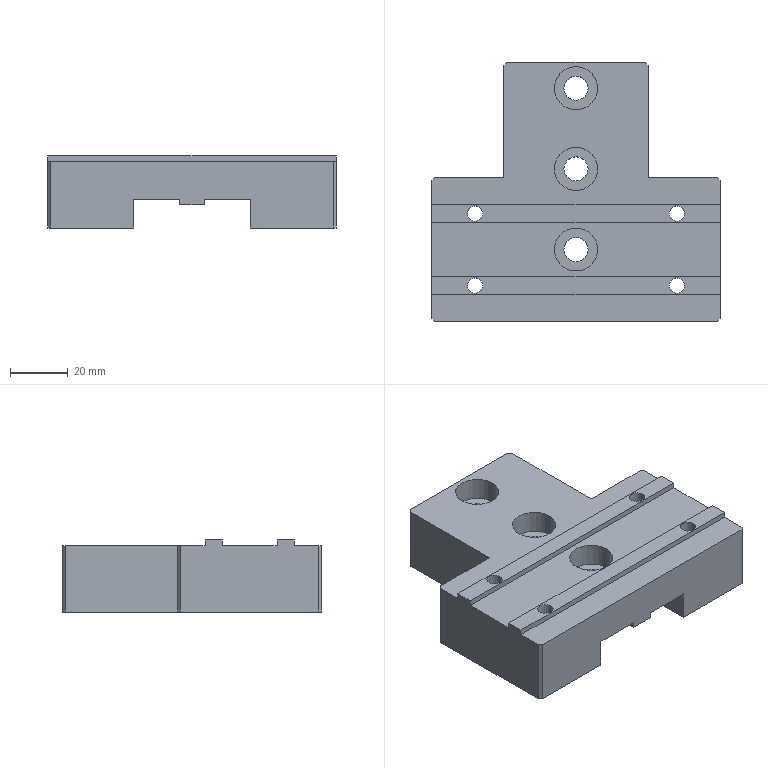Part | STEP file | CON-012 | 1 solid | 76 faces | box 100 x 90 x 25 mm | volume 119624 mm3 | plane 48 | cylinder 28 | commonest cylinder face diameters 5.3 x8 10 x8 8.4 x6 15 x6